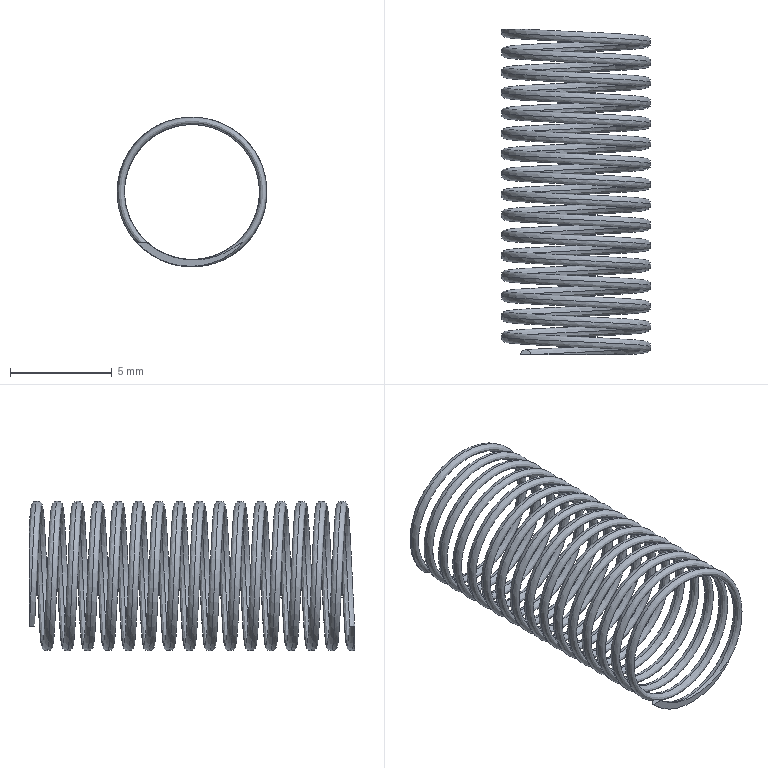Part | STEP file | Guide wheel mechanism revised.sldasm-Part-433 | 1 solid | 6 faces | box 7.362 x 16 x 7.362 mm | volume 48.535 mm3 | plane 4 | spline 2